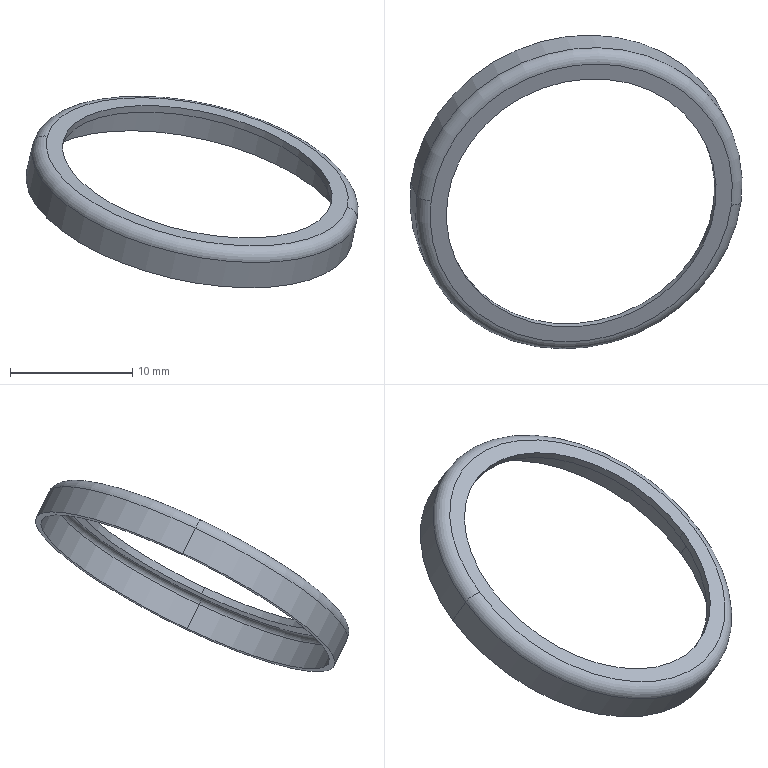Part | SolidWorks | features BaseBody 1 | 1 solid | 13 faces | box 27.136 x 25.603 x 15.645 mm | volume 211.754 mm3 | cylinder 6 | torus 4 | plane 3 | commonest cylinder face diameters 22.5 x2 26.2 x2 27.2 x2
STEP:
#1=CARTESIAN_POINT('',(1972.198,-232.396,967.631));
#2=VERTEX_POINT('',#1);
#3=CARTESIAN_POINT('',(1950.304,-232.096,972.809));
#4=VERTEX_POINT('',#3);
#5=CARTESIAN_POINT('',(1961.251,-232.246,970.22));
#6=DIRECTION('',(-0.2015,0.436,-0.8771));
#7=DIRECTION('',(0.9077,0.4197,0.0001618));
#8=AXIS2_PLACEMENT_3D('',#5,#6,#7);
#9=CIRCLE('',#8,11.25);
#10=EDGE_CURVE('',#2,#4,#9,.T.);
#11=ORIENTED_EDGE('',*,*,#10,.F.);
#12=CARTESIAN_POINT('',(1972.077,-232.134,967.105));
#13=VERTEX_POINT('',#12);
#14=CARTESIAN_POINT('',(1972.138,-232.265,967.368));
#15=DIRECTION('',(-0.2015,0.436,-0.8771));
#16=VECTOR('',#15,1000.);
#17=LINE('',#14,#16);
#18=EDGE_CURVE('',#2,#13,#17,.T.);
#19=ORIENTED_EDGE('',*,*,#18,.T.);
#20=CARTESIAN_POINT('',(1950.183,-231.835,972.283));
#21=VERTEX_POINT('',#20);
#22=CARTESIAN_POINT('',(1961.13,-231.985,969.694));
#23=DIRECTION('',(-0.2015,0.436,-0.8771));
#24=DIRECTION('',(0.9077,0.4197,0.0001618));
#25=AXIS2_PLACEMENT_3D('',#22,#23,#24);
#26=CIRCLE('',#25,11.25);
#27=EDGE_CURVE('',#13,#21,#26,.T.);
#28=ORIENTED_EDGE('',*,*,#27,.T.);
#29=CARTESIAN_POINT('',(1950.244,-231.966,972.546));
#30=DIRECTION('',(0.2015,-0.436,0.8771));
#31=VECTOR('',#30,1000.);
#32=LINE('',#29,#31);
#33=EDGE_CURVE('',#21,#4,#32,.T.);
#34=ORIENTED_EDGE('',*,*,#33,.T.);
#35=EDGE_LOOP('',(#11,#19,#28,#34));
#36=FACE_OUTER_BOUND('',#35,.T.);
#37=CARTESIAN_POINT('',(1960.914,-231.516,968.751));
#38=DIRECTION('',(-0.2015,0.436,-0.8771));
#39=DIRECTION('',(-0.9731,0.01332,0.2301));
#40=AXIS2_PLACEMENT_3D('',#37,#38,#39);
#41=CYLINDRICAL_SURFACE('',#40,11.25);
#42=ADVANCED_FACE('',(#36),#41,.F.);
#43=CARTESIAN_POINT('',(1961.251,-232.246,970.22));
#44=DIRECTION('',(-0.2015,0.436,-0.8771));
#45=DIRECTION('',(0.9077,0.4197,0.0001618));
#46=AXIS2_PLACEMENT_3D('',#43,#44,#45);
#47=CIRCLE('',#46,11.25);
#48=EDGE_CURVE('',#4,#2,#47,.T.);
#49=ORIENTED_EDGE('',*,*,#48,.F.);
#50=ORIENTED_EDGE('',*,*,#33,.F.);
#51=CARTESIAN_POINT('',(1961.13,-231.985,969.694));
#52=DIRECTION('',(-0.2015,0.436,-0.8771));
#53=DIRECTION('',(0.9077,0.4197,0.0001618));
#54=AXIS2_PLACEMENT_3D('',#51,#52,#53);
#55=CIRCLE('',#54,11.25);
#56=EDGE_CURVE('',#21,#13,#55,.T.);
#57=ORIENTED_EDGE('',*,*,#56,.T.);
#58=ORIENTED_EDGE('',*,*,#18,.F.);
#59=EDGE_LOOP('',(#49,#50,#57,#58));
#60=FACE_OUTER_BOUND('',#59,.T.);
#61=CARTESIAN_POINT('',(1960.914,-231.516,968.751));
#62=DIRECTION('',(-0.2015,0.436,-0.8771));
#63=DIRECTION('',(-0.9731,0.01332,0.2301));
#64=AXIS2_PLACEMENT_3D('',#61,#62,#63);
#65=CYLINDRICAL_SURFACE('',#64,11.25);
#66=ADVANCED_FACE('',(#60),#65,.F.);
#67=CARTESIAN_POINT('',(1973.391,-232.152,966.794));
#68=VERTEX_POINT('',#67);
#69=CARTESIAN_POINT('',(1948.87,-231.817,972.593));
#70=VERTEX_POINT('',#69);
#71=CARTESIAN_POINT('',(1961.13,-231.985,969.694));
#72=DIRECTION('',(-0.2015,0.436,-0.8771));
#73=DIRECTION('',(0.9077,0.4197,0.0001618));
#74=AXIS2_PLACEMENT_3D('',#71,#72,#73);
#75=CIRCLE('',#74,12.6);
#76=EDGE_CURVE('',#68,#70,#75,.T.);
#77=ORIENTED_EDGE('',*,*,#76,.F.);
#78=CARTESIAN_POINT('',(1973.777,-231.941,966.24));
#79=VERTEX_POINT('',#78);
#80=CARTESIAN_POINT('',(1973.29,-231.934,966.356));
#81=DIRECTION('',(0.112,0.8998,0.4216));
#82=DIRECTION('',(0.9731,-0.01332,-0.2301));
#83=AXIS2_PLACEMENT_3D('',#80,#81,#82);
#84=CIRCLE('',#83,0.5);
#85=EDGE_CURVE('',#68,#79,#84,.T.);
#86=ORIENTED_EDGE('',*,*,#85,.T.);
#87=CARTESIAN_POINT('',(1948.282,-231.592,972.27));
#88=VERTEX_POINT('',#87);
#89=CARTESIAN_POINT('',(1961.03,-231.767,969.255));
#90=DIRECTION('',(-0.2015,0.436,-0.8771));
#91=DIRECTION('',(0.9077,0.4197,0.0001618));
#92=AXIS2_PLACEMENT_3D('',#89,#90,#91);
#93=CIRCLE('',#92,13.1);
#94=EDGE_CURVE('',#79,#88,#93,.T.);
#95=ORIENTED_EDGE('',*,*,#94,.T.);
#96=CARTESIAN_POINT('',(1948.769,-231.599,972.155));
#97=DIRECTION('',(0.112,0.8998,0.4216));
#98=DIRECTION('',(0.9731,-0.01332,-0.2301));
#99=AXIS2_PLACEMENT_3D('',#96,#97,#98);
#100=CIRCLE('',#99,0.5);
#101=EDGE_CURVE('',#88,#70,#100,.T.);
#102=ORIENTED_EDGE('',*,*,#101,.T.);
#103=EDGE_LOOP('',(#77,#86,#95,#102));
#104=FACE_OUTER_BOUND('',#103,.T.);
#105=CARTESIAN_POINT('',(1961.03,-231.767,969.255));
#106=DIRECTION('',(-0.2015,0.436,-0.8771));
#107=DIRECTION('',(-0.9731,0.01332,0.2301));
#108=AXIS2_PLACEMENT_3D('',#105,#106,#107);
#109=TOROIDAL_SURFACE('',#108,12.6,0.5);
#110=ADVANCED_FACE('',(#104),#109,.F.);
#111=CARTESIAN_POINT('',(1961.13,-231.985,969.694));
#112=DIRECTION('',(-0.2015,0.436,-0.8771));
#113=DIRECTION('',(0.9077,0.4197,0.0001618));
#114=AXIS2_PLACEMENT_3D('',#111,#112,#113);
#115=CIRCLE('',#114,12.6);
#116=EDGE_CURVE('',#70,#68,#115,.T.);
#117=ORIENTED_EDGE('',*,*,#116,.F.);
#118=ORIENTED_EDGE('',*,*,#101,.F.);
#119=CARTESIAN_POINT('',(1961.03,-231.767,969.255));
#120=DIRECTION('',(-0.2015,0.436,-0.8771));
#121=DIRECTION('',(0.9077,0.4197,0.0001618));
#122=AXIS2_PLACEMENT_3D('',#119,#120,#121);
#123=CIRCLE('',#122,13.1);
#124=EDGE_CURVE('',#88,#79,#123,.T.);
#125=ORIENTED_EDGE('',*,*,#124,.T.);
#126=ORIENTED_EDGE('',*,*,#85,.F.);
#127=EDGE_LOOP('',(#117,#118,#125,#126));
#128=FACE_OUTER_BOUND('',#127,.T.);
#129=CARTESIAN_POINT('',(1961.03,-231.767,969.255));
#130=DIRECTION('',(-0.2015,0.436,-0.8771));
#131=DIRECTION('',(-0.9731,0.01332,0.2301));
#132=AXIS2_PLACEMENT_3D('',#129,#130,#131);
#133=TOROIDAL_SURFACE('',#132,12.6,0.5);
#134=ADVANCED_FACE('',(#128),#133,.F.);
#135=ORIENTED_EDGE('',*,*,#94,.F.);
#136=CARTESIAN_POINT('',(1973.323,-230.96,964.267));
#137=VERTEX_POINT('',#136);
#138=CARTESIAN_POINT('',(1973.55,-231.45,965.254));
#139=DIRECTION('',(0.2015,-0.436,0.8771));
#140=VECTOR('',#139,1000.);
#141=LINE('',#138,#140);
#142=EDGE_CURVE('',#137,#79,#141,.T.);
#143=ORIENTED_EDGE('',*,*,#142,.F.);
#144=CARTESIAN_POINT('',(1947.829,-230.611,970.296));
#145=VERTEX_POINT('',#144);
#146=CARTESIAN_POINT('',(1960.576,-230.785,967.282));
#147=DIRECTION('',(-0.2015,0.436,-0.8771));
#148=DIRECTION('',(0.9077,0.4197,0.0001618));
#149=AXIS2_PLACEMENT_3D('',#146,#147,#148);
#150=CIRCLE('',#149,13.1);
#151=EDGE_CURVE('',#137,#145,#150,.T.);
#152=ORIENTED_EDGE('',*,*,#151,.T.);
#153=CARTESIAN_POINT('',(1948.056,-231.102,971.283));
#154=DIRECTION('',(-0.2015,0.436,-0.8771));
#155=VECTOR('',#154,1000.);
#156=LINE('',#153,#155);
#157=EDGE_CURVE('',#88,#145,#156,.T.);
#158=ORIENTED_EDGE('',*,*,#157,.F.);
#159=EDGE_LOOP('',(#135,#143,#152,#158));
#160=FACE_OUTER_BOUND('',#159,.T.);
#161=CARTESIAN_POINT('',(1960.914,-231.516,968.751));
#162=DIRECTION('',(-0.2015,0.436,-0.8771));
#163=DIRECTION('',(-0.9731,0.01332,0.2301));
#164=AXIS2_PLACEMENT_3D('',#161,#162,#163);
#165=CYLINDRICAL_SURFACE('',#164,13.1);
#166=ADVANCED_FACE('',(#160),#165,.F.);
#167=ORIENTED_EDGE('',*,*,#124,.F.);
#168=ORIENTED_EDGE('',*,*,#157,.T.);
#169=CARTESIAN_POINT('',(1960.576,-230.785,967.282));
#170=DIRECTION('',(-0.2015,0.436,-0.8771));
#171=DIRECTION('',(0.9077,0.4197,0.0001618));
#172=AXIS2_PLACEMENT_3D('',#169,#170,#171);
#173=CIRCLE('',#172,13.1);
#174=EDGE_CURVE('',#145,#137,#173,.T.);
#175=ORIENTED_EDGE('',*,*,#174,.T.);
#176=ORIENTED_EDGE('',*,*,#142,.T.);
#177=EDGE_LOOP('',(#167,#168,#175,#176));
#178=FACE_OUTER_BOUND('',#177,.T.);
#179=CARTESIAN_POINT('',(1960.914,-231.516,968.751));
#180=DIRECTION('',(-0.2015,0.436,-0.8771));
#181=DIRECTION('',(-0.9731,0.01332,0.2301));
#182=AXIS2_PLACEMENT_3D('',#179,#180,#181);
#183=CYLINDRICAL_SURFACE('',#182,13.1);
#184=ADVANCED_FACE('',(#178),#183,.F.);
#185=CARTESIAN_POINT('',(1973.81,-230.967,964.152));
#186=VERTEX_POINT('',#185);
#187=CARTESIAN_POINT('',(1947.343,-230.604,970.412));
#188=VERTEX_POINT('',#187);
#189=CARTESIAN_POINT('',(1960.576,-230.785,967.282));
#190=DIRECTION('',(-0.2015,0.436,-0.8771));
#191=DIRECTION('',(0.9077,0.4197,0.0001618));
#192=AXIS2_PLACEMENT_3D('',#189,#190,#191);
#193=CIRCLE('',#192,13.6);
#194=EDGE_CURVE('',#186,#188,#193,.T.);
#195=ORIENTED_EDGE('',*,*,#194,.F.);
#196=CARTESIAN_POINT('',(1974.283,-231.991,966.213));
#197=VERTEX_POINT('',#196);
#198=CARTESIAN_POINT('',(1974.047,-231.479,965.183));
#199=DIRECTION('',(0.2015,-0.436,0.8771));
#200=VECTOR('',#199,1000.);
#201=LINE('',#198,#200);
#202=EDGE_CURVE('',#186,#197,#201,.T.);
#203=ORIENTED_EDGE('',*,*,#202,.T.);
#204=CARTESIAN_POINT('',(1947.816,-231.629,972.473));
#205=VERTEX_POINT('',#204);
#206=CARTESIAN_POINT('',(1961.05,-231.81,969.343));
#207=DIRECTION('',(-0.2015,0.436,-0.8771));
#208=DIRECTION('',(0.9077,0.4197,0.0001618));
#209=AXIS2_PLACEMENT_3D('',#206,#207,#208);
#210=CIRCLE('',#209,13.6);
#211=EDGE_CURVE('',#197,#205,#210,.T.);
#212=ORIENTED_EDGE('',*,*,#211,.T.);
#213=CARTESIAN_POINT('',(1947.579,-231.117,971.442));
#214=DIRECTION('',(-0.2015,0.436,-0.8771));
#215=VECTOR('',#214,1000.);
#216=LINE('',#213,#215);
#217=EDGE_CURVE('',#205,#188,#216,.T.);
#218=ORIENTED_EDGE('',*,*,#217,.T.);
#219=EDGE_LOOP('',(#195,#203,#212,#218));
#220=FACE_OUTER_BOUND('',#219,.T.);
#221=CARTESIAN_POINT('',(1960.914,-231.516,968.751));
#222=DIRECTION('',(-0.2015,0.436,-0.8771));
#223=DIRECTION('',(-0.9731,0.01332,0.2301));
#224=AXIS2_PLACEMENT_3D('',#221,#222,#223);
#225=CYLINDRICAL_SURFACE('',#224,13.6);
#226=ADVANCED_FACE('',(#220),#225,.T.);
#227=CARTESIAN_POINT('',(1960.576,-230.785,967.282));
#228=DIRECTION('',(-0.2015,0.436,-0.8771));
#229=DIRECTION('',(0.9077,0.4197,0.0001618));
#230=AXIS2_PLACEMENT_3D('',#227,#228,#229);
#231=CIRCLE('',#230,13.6);
#232=EDGE_CURVE('',#188,#186,#231,.T.);
#233=ORIENTED_EDGE('',*,*,#232,.F.);
#234=ORIENTED_EDGE('',*,*,#217,.F.);
#235=CARTESIAN_POINT('',(1961.05,-231.81,969.343));
#236=DIRECTION('',(-0.2015,0.436,-0.8771));
#237=DIRECTION('',(0.9077,0.4197,0.0001618));
#238=AXIS2_PLACEMENT_3D('',#235,#236,#237);
#239=CIRCLE('',#238,13.6);
#240=EDGE_CURVE('',#205,#197,#239,.T.);
#241=ORIENTED_EDGE('',*,*,#240,.T.);
#242=ORIENTED_EDGE('',*,*,#202,.F.);
#243=EDGE_LOOP('',(#233,#234,#241,#242));
#244=FACE_OUTER_BOUND('',#243,.T.);
#245=CARTESIAN_POINT('',(1960.914,-231.516,968.751));
#246=DIRECTION('',(-0.2015,0.436,-0.8771));
#247=DIRECTION('',(-0.9731,0.01332,0.2301));
#248=AXIS2_PLACEMENT_3D('',#245,#246,#247);
#249=CYLINDRICAL_SURFACE('',#248,13.6);
#250=ADVANCED_FACE('',(#244),#249,.T.);
#251=ORIENTED_EDGE('',*,*,#211,.F.);
#252=CARTESIAN_POINT('',(1973.512,-232.414,967.32));
#253=VERTEX_POINT('',#252);
#254=CARTESIAN_POINT('',(1973.31,-231.978,966.443));
#255=DIRECTION('',(0.112,0.8998,0.4216));
#256=DIRECTION('',(0.9731,-0.01332,-0.2301));
#257=AXIS2_PLACEMENT_3D('',#254,#255,#256);
#258=CIRCLE('',#257,1.);
#259=EDGE_CURVE('',#253,#197,#258,.T.);
#260=ORIENTED_EDGE('',*,*,#259,.F.);
#261=CARTESIAN_POINT('',(1948.991,-232.078,973.12));
#262=VERTEX_POINT('',#261);
#263=CARTESIAN_POINT('',(1961.251,-232.246,970.22));
#264=DIRECTION('',(-0.2015,0.436,-0.8771));
#265=DIRECTION('',(0.9077,0.4197,0.0001618));
#266=AXIS2_PLACEMENT_3D('',#263,#264,#265);
#267=CIRCLE('',#266,12.6);
#268=EDGE_CURVE('',#253,#262,#267,.T.);
#269=ORIENTED_EDGE('',*,*,#268,.T.);
#270=CARTESIAN_POINT('',(1948.789,-231.642,972.243));
#271=DIRECTION('',(0.112,0.8998,0.4216));
#272=DIRECTION('',(0.9731,-0.01332,-0.2301));
#273=AXIS2_PLACEMENT_3D('',#270,#271,#272);
#274=CIRCLE('',#273,1.);
#275=EDGE_CURVE('',#205,#262,#274,.T.);
#276=ORIENTED_EDGE('',*,*,#275,.F.);
#277=EDGE_LOOP('',(#251,#260,#269,#276));
#278=FACE_OUTER_BOUND('',#277,.T.);
#279=CARTESIAN_POINT('',(1961.05,-231.81,969.343));
#280=DIRECTION('',(-0.2015,0.436,-0.8771));
#281=DIRECTION('',(-0.9731,0.01332,0.2301));
#282=AXIS2_PLACEMENT_3D('',#279,#280,#281);
#283=TOROIDAL_SURFACE('',#282,12.6,1.);
#284=ADVANCED_FACE('',(#278),#283,.T.);
#285=ORIENTED_EDGE('',*,*,#240,.F.);
#286=ORIENTED_EDGE('',*,*,#275,.T.);
#287=CARTESIAN_POINT('',(1961.251,-232.246,970.22));
#288=DIRECTION('',(-0.2015,0.436,-0.8771));
#289=DIRECTION('',(0.9077,0.4197,0.0001618));
#290=AXIS2_PLACEMENT_3D('',#287,#288,#289);
#291=CIRCLE('',#290,12.6);
#292=EDGE_CURVE('',#262,#253,#291,.T.);
#293=ORIENTED_EDGE('',*,*,#292,.T.);
#294=ORIENTED_EDGE('',*,*,#259,.T.);
#295=EDGE_LOOP('',(#285,#286,#293,#294));
#296=FACE_OUTER_BOUND('',#295,.T.);
#297=CARTESIAN_POINT('',(1961.05,-231.81,969.343));
#298=DIRECTION('',(-0.2015,0.436,-0.8771));
#299=DIRECTION('',(-0.9731,0.01332,0.2301));
#300=AXIS2_PLACEMENT_3D('',#297,#298,#299);
#301=TOROIDAL_SURFACE('',#300,12.6,1.);
#302=ADVANCED_FACE('',(#296),#301,.T.);
#303=ORIENTED_EDGE('',*,*,#116,.T.);
#304=ORIENTED_EDGE('',*,*,#76,.T.);
#305=EDGE_LOOP('',(#303,#304));
#306=FACE_OUTER_BOUND('',#305,.T.);
#307=ORIENTED_EDGE('',*,*,#27,.F.);
#308=ORIENTED_EDGE('',*,*,#56,.F.);
#309=EDGE_LOOP('',(#307,#308));
#310=FACE_BOUND('',#309,.T.);
#311=CARTESIAN_POINT('',(1971.341,-227.263,969.696));
#312=DIRECTION('',(-0.2015,0.436,-0.8771));
#313=DIRECTION('',(-0.9077,-0.4197,-0.0001618));
#314=AXIS2_PLACEMENT_3D('',#311,#312,#313);
#315=PLANE('',#314);
#316=ADVANCED_FACE('',(#306,#310),#315,.T.);
#317=ORIENTED_EDGE('',*,*,#232,.T.);
#318=ORIENTED_EDGE('',*,*,#194,.T.);
#319=EDGE_LOOP('',(#317,#318));
#320=FACE_OUTER_BOUND('',#319,.T.);
#321=ORIENTED_EDGE('',*,*,#151,.F.);
#322=ORIENTED_EDGE('',*,*,#174,.F.);
#323=EDGE_LOOP('',(#321,#322));
#324=FACE_BOUND('',#323,.T.);
#325=CARTESIAN_POINT('',(1972.92,-225.077,967.284));
#326=DIRECTION('',(-0.2015,0.436,-0.8771));
#327=DIRECTION('',(-0.9077,-0.4197,-0.0001618));
#328=AXIS2_PLACEMENT_3D('',#325,#326,#327);
#329=PLANE('',#328);
#330=ADVANCED_FACE('',(#320,#324),#329,.T.);
#331=ORIENTED_EDGE('',*,*,#268,.F.);
#332=ORIENTED_EDGE('',*,*,#292,.F.);
#333=EDGE_LOOP('',(#331,#332));
#334=FACE_OUTER_BOUND('',#333,.T.);
#335=ORIENTED_EDGE('',*,*,#48,.T.);
#336=ORIENTED_EDGE('',*,*,#10,.T.);
#337=EDGE_LOOP('',(#335,#336));
#338=FACE_BOUND('',#337,.T.);
#339=CARTESIAN_POINT('',(1971.462,-227.524,970.222));
#340=DIRECTION('',(-0.2015,0.436,-0.8771));
#341=DIRECTION('',(-0.9077,-0.4197,-0.0001618));
#342=AXIS2_PLACEMENT_3D('',#339,#340,#341);
#343=PLANE('',#342);
#344=ADVANCED_FACE('',(#334,#338),#343,.F.);
#345=CLOSED_SHELL('',(#42,#66,#110,#134,#166,#184,#226,#250,#284,#302,#316,#330,#344));
#346=MANIFOLD_SOLID_BREP('',#345);
#347=CARTESIAN_POINT('',(0.,0.,0.));
#348=DIRECTION('',(0.,0.,1.));
#349=DIRECTION('',(1.,0.,0.));
#350=AXIS2_PLACEMENT_3D('',#347,#348,#349);
#351=(LENGTH_UNIT()NAMED_UNIT(*)SI_UNIT(.MILLI.,.METRE.));
#352=UNCERTAINTY_MEASURE_WITH_UNIT(LENGTH_MEASURE(0.00001),#351,'','');
#353=(NAMED_UNIT(*)PLANE_ANGLE_UNIT()SI_UNIT($,.RADIAN.));
#354=(NAMED_UNIT(*)SI_UNIT($,.STERADIAN.)SOLID_ANGLE_UNIT());
#355=(GEOMETRIC_REPRESENTATION_CONTEXT(3)GLOBAL_UNCERTAINTY_ASSIGNED_CONTEXT((#352))GLOBAL_UNIT_ASSIGNED_CONTEXT((#351,#353,#354))REPRESENTATION_CONTEXT('',''));
#356=ADVANCED_BREP_SHAPE_REPRESENTATION('',(#346,#350),#355);